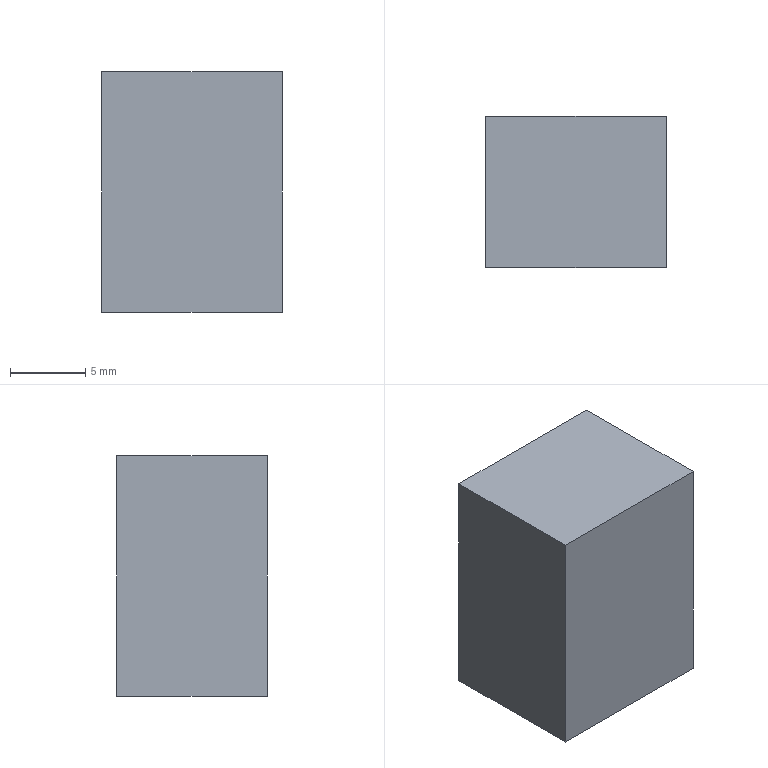Part | SolidWorks | features BaseBody 1 | 1 solid | 6 faces | box 12 x 10 x 16 mm | volume 1920 mm3 | plane 6
STEP:
#1=CARTESIAN_POINT('',(-6.,-5.,8.));
#2=VERTEX_POINT('',#1);
#3=CARTESIAN_POINT('',(6.,-5.,8.));
#4=VERTEX_POINT('',#3);
#5=CARTESIAN_POINT('',(-6.,-5.,8.));
#6=DIRECTION('',(1.,0.,0.));
#7=VECTOR('',#6,1000.);
#8=LINE('',#5,#7);
#9=EDGE_CURVE('',#2,#4,#8,.T.);
#10=ORIENTED_EDGE('',*,*,#9,.F.);
#11=CARTESIAN_POINT('',(-6.,-5.,-8.));
#12=VERTEX_POINT('',#11);
#13=CARTESIAN_POINT('',(-6.,-5.,-8.));
#14=DIRECTION('',(0.,0.,1.));
#15=VECTOR('',#14,1000.);
#16=LINE('',#13,#15);
#17=EDGE_CURVE('',#12,#2,#16,.T.);
#18=ORIENTED_EDGE('',*,*,#17,.F.);
#19=CARTESIAN_POINT('',(6.,-5.,-8.));
#20=VERTEX_POINT('',#19);
#21=CARTESIAN_POINT('',(-6.,-5.,-8.));
#22=DIRECTION('',(-1.,0.,0.));
#23=VECTOR('',#22,1000.);
#24=LINE('',#21,#23);
#25=EDGE_CURVE('',#20,#12,#24,.T.);
#26=ORIENTED_EDGE('',*,*,#25,.F.);
#27=CARTESIAN_POINT('',(6.,-5.,-8.));
#28=DIRECTION('',(0.,0.,-1.));
#29=VECTOR('',#28,1000.);
#30=LINE('',#27,#29);
#31=EDGE_CURVE('',#4,#20,#30,.T.);
#32=ORIENTED_EDGE('',*,*,#31,.F.);
#33=EDGE_LOOP('',(#10,#18,#26,#32));
#34=FACE_OUTER_BOUND('',#33,.T.);
#35=CARTESIAN_POINT('',(-6.,-5.,-8.));
#36=DIRECTION('',(0.,1.,0.));
#37=DIRECTION('',(0.,0.,1.));
#38=AXIS2_PLACEMENT_3D('',#35,#36,#37);
#39=PLANE('',#38);
#40=ADVANCED_FACE('',(#34),#39,.F.);
#41=CARTESIAN_POINT('',(6.,5.,-8.));
#42=VERTEX_POINT('',#41);
#43=CARTESIAN_POINT('',(6.,5.,8.));
#44=VERTEX_POINT('',#43);
#45=CARTESIAN_POINT('',(6.,5.,-8.));
#46=DIRECTION('',(0.,0.,1.));
#47=VECTOR('',#46,1000.);
#48=LINE('',#45,#47);
#49=EDGE_CURVE('',#42,#44,#48,.T.);
#50=ORIENTED_EDGE('',*,*,#49,.T.);
#51=CARTESIAN_POINT('',(6.,-5.,8.));
#52=DIRECTION('',(0.,-1.,0.));
#53=VECTOR('',#52,1000.);
#54=LINE('',#51,#53);
#55=EDGE_CURVE('',#44,#4,#54,.T.);
#56=ORIENTED_EDGE('',*,*,#55,.T.);
#57=ORIENTED_EDGE('',*,*,#31,.T.);
#58=CARTESIAN_POINT('',(6.,-5.,-8.));
#59=DIRECTION('',(0.,1.,0.));
#60=VECTOR('',#59,1000.);
#61=LINE('',#58,#60);
#62=EDGE_CURVE('',#20,#42,#61,.T.);
#63=ORIENTED_EDGE('',*,*,#62,.T.);
#64=EDGE_LOOP('',(#50,#56,#57,#63));
#65=FACE_OUTER_BOUND('',#64,.T.);
#66=CARTESIAN_POINT('',(6.,-5.,-8.));
#67=DIRECTION('',(1.,0.,0.));
#68=DIRECTION('',(0.,0.,-1.));
#69=AXIS2_PLACEMENT_3D('',#66,#67,#68);
#70=PLANE('',#69);
#71=ADVANCED_FACE('',(#65),#70,.T.);
#72=ORIENTED_EDGE('',*,*,#55,.F.);
#73=CARTESIAN_POINT('',(-6.,5.,8.));
#74=VERTEX_POINT('',#73);
#75=CARTESIAN_POINT('',(-6.,5.,8.));
#76=DIRECTION('',(-1.,0.,0.));
#77=VECTOR('',#76,1000.);
#78=LINE('',#75,#77);
#79=EDGE_CURVE('',#44,#74,#78,.T.);
#80=ORIENTED_EDGE('',*,*,#79,.T.);
#81=CARTESIAN_POINT('',(-6.,-5.,8.));
#82=DIRECTION('',(0.,-1.,0.));
#83=VECTOR('',#82,1000.);
#84=LINE('',#81,#83);
#85=EDGE_CURVE('',#74,#2,#84,.T.);
#86=ORIENTED_EDGE('',*,*,#85,.T.);
#87=ORIENTED_EDGE('',*,*,#9,.T.);
#88=EDGE_LOOP('',(#72,#80,#86,#87));
#89=FACE_OUTER_BOUND('',#88,.T.);
#90=CARTESIAN_POINT('',(-6.,-5.,8.));
#91=DIRECTION('',(0.,0.,1.));
#92=DIRECTION('',(1.,0.,0.));
#93=AXIS2_PLACEMENT_3D('',#90,#91,#92);
#94=PLANE('',#93);
#95=ADVANCED_FACE('',(#89),#94,.T.);
#96=CARTESIAN_POINT('',(-6.,5.,-8.));
#97=VERTEX_POINT('',#96);
#98=CARTESIAN_POINT('',(-6.,5.,-8.));
#99=DIRECTION('',(0.,0.,1.));
#100=VECTOR('',#99,1000.);
#101=LINE('',#98,#100);
#102=EDGE_CURVE('',#97,#74,#101,.T.);
#103=ORIENTED_EDGE('',*,*,#102,.F.);
#104=CARTESIAN_POINT('',(-6.,-5.,-8.));
#105=DIRECTION('',(0.,1.,0.));
#106=VECTOR('',#105,1000.);
#107=LINE('',#104,#106);
#108=EDGE_CURVE('',#12,#97,#107,.T.);
#109=ORIENTED_EDGE('',*,*,#108,.F.);
#110=ORIENTED_EDGE('',*,*,#17,.T.);
#111=ORIENTED_EDGE('',*,*,#85,.F.);
#112=EDGE_LOOP('',(#103,#109,#110,#111));
#113=FACE_OUTER_BOUND('',#112,.T.);
#114=CARTESIAN_POINT('',(-6.,-5.,-8.));
#115=DIRECTION('',(1.,0.,0.));
#116=DIRECTION('',(0.,0.,-1.));
#117=AXIS2_PLACEMENT_3D('',#114,#115,#116);
#118=PLANE('',#117);
#119=ADVANCED_FACE('',(#113),#118,.F.);
#120=ORIENTED_EDGE('',*,*,#62,.F.);
#121=ORIENTED_EDGE('',*,*,#25,.T.);
#122=ORIENTED_EDGE('',*,*,#108,.T.);
#123=CARTESIAN_POINT('',(-6.,5.,-8.));
#124=DIRECTION('',(-1.,0.,0.));
#125=VECTOR('',#124,1000.);
#126=LINE('',#123,#125);
#127=EDGE_CURVE('',#42,#97,#126,.T.);
#128=ORIENTED_EDGE('',*,*,#127,.F.);
#129=EDGE_LOOP('',(#120,#121,#122,#128));
#130=FACE_OUTER_BOUND('',#129,.T.);
#131=CARTESIAN_POINT('',(-6.,-5.,-8.));
#132=DIRECTION('',(0.,0.,1.));
#133=DIRECTION('',(1.,0.,0.));
#134=AXIS2_PLACEMENT_3D('',#131,#132,#133);
#135=PLANE('',#134);
#136=ADVANCED_FACE('',(#130),#135,.F.);
#137=ORIENTED_EDGE('',*,*,#79,.F.);
#138=ORIENTED_EDGE('',*,*,#49,.F.);
#139=ORIENTED_EDGE('',*,*,#127,.T.);
#140=ORIENTED_EDGE('',*,*,#102,.T.);
#141=EDGE_LOOP('',(#137,#138,#139,#140));
#142=FACE_OUTER_BOUND('',#141,.T.);
#143=CARTESIAN_POINT('',(-6.,5.,-8.));
#144=DIRECTION('',(0.,1.,0.));
#145=DIRECTION('',(0.,0.,1.));
#146=AXIS2_PLACEMENT_3D('',#143,#144,#145);
#147=PLANE('',#146);
#148=ADVANCED_FACE('',(#142),#147,.T.);
#149=CLOSED_SHELL('',(#40,#71,#95,#119,#136,#148));
#150=MANIFOLD_SOLID_BREP('',#149);
#151=CARTESIAN_POINT('',(0.,0.,0.));
#152=DIRECTION('',(0.,0.,1.));
#153=DIRECTION('',(1.,0.,0.));
#154=AXIS2_PLACEMENT_3D('',#151,#152,#153);
#155=(LENGTH_UNIT()NAMED_UNIT(*)SI_UNIT(.MILLI.,.METRE.));
#156=UNCERTAINTY_MEASURE_WITH_UNIT(LENGTH_MEASURE(0.00001),#155,'','');
#157=(NAMED_UNIT(*)PLANE_ANGLE_UNIT()SI_UNIT($,.RADIAN.));
#158=(NAMED_UNIT(*)SI_UNIT($,.STERADIAN.)SOLID_ANGLE_UNIT());
#159=(GEOMETRIC_REPRESENTATION_CONTEXT(3)GLOBAL_UNCERTAINTY_ASSIGNED_CONTEXT((#156))GLOBAL_UNIT_ASSIGNED_CONTEXT((#155,#157,#158))REPRESENTATION_CONTEXT('',''));
#160=ADVANCED_BREP_SHAPE_REPRESENTATION('',(#150,#154),#159);